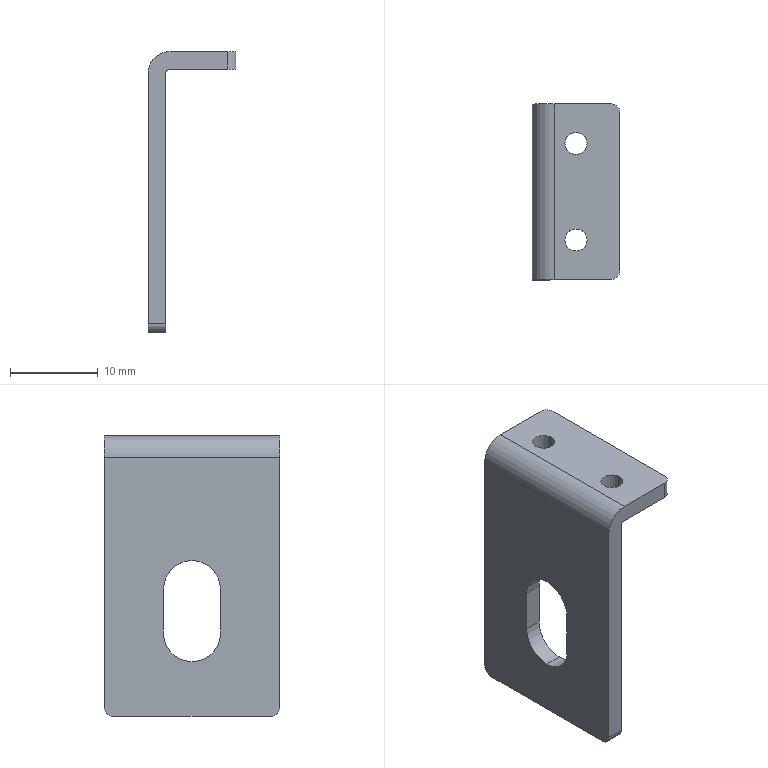Part | SolidWorks | features BaseBody 1, HoleWzd 1 | 1 solid | 23 faces | box 10 x 20 x 32 mm | volume 1421 mm3 | cylinder 13 | plane 10 | commonest cylinder face diameters 2 x4 2.51 x4 6.5 x3 1 x1 5 x1
STEP:
#1=CARTESIAN_POINT('',(4.255,15.5,0.));
#2=VERTEX_POINT('',#1);
#3=CARTESIAN_POINT('',(1.745,15.5,0.));
#4=VERTEX_POINT('',#3);
#5=CARTESIAN_POINT('',(3.,15.5,0.));
#6=DIRECTION('',(0.,0.,-1.));
#7=DIRECTION('',(-1.,0.,0.));
#8=AXIS2_PLACEMENT_3D('',#5,#6,#7);
#9=CIRCLE('',#8,1.255);
#10=EDGE_CURVE('',#2,#4,#9,.T.);
#11=ORIENTED_EDGE('',*,*,#10,.T.);
#12=CARTESIAN_POINT('',(1.745,15.5,2.));
#13=VERTEX_POINT('',#12);
#14=CARTESIAN_POINT('',(1.745,15.5,2.));
#15=DIRECTION('',(0.,0.,1.));
#16=VECTOR('',#15,1000.);
#17=LINE('',#14,#16);
#18=EDGE_CURVE('',#4,#13,#17,.T.);
#19=ORIENTED_EDGE('',*,*,#18,.T.);
#20=CARTESIAN_POINT('',(4.255,15.5,2.));
#21=VERTEX_POINT('',#20);
#22=CARTESIAN_POINT('',(3.,15.5,2.));
#23=DIRECTION('',(0.,0.,1.));
#24=DIRECTION('',(1.,0.,0.));
#25=AXIS2_PLACEMENT_3D('',#22,#23,#24);
#26=CIRCLE('',#25,1.255);
#27=EDGE_CURVE('',#13,#21,#26,.T.);
#28=ORIENTED_EDGE('',*,*,#27,.T.);
#29=CARTESIAN_POINT('',(4.255,15.5,2.));
#30=DIRECTION('',(0.,0.,1.));
#31=VECTOR('',#30,1000.);
#32=LINE('',#29,#31);
#33=EDGE_CURVE('',#2,#21,#32,.T.);
#34=ORIENTED_EDGE('',*,*,#33,.F.);
#35=EDGE_LOOP('',(#11,#19,#28,#34));
#36=FACE_OUTER_BOUND('',#35,.T.);
#37=CARTESIAN_POINT('',(3.,15.5,2.));
#38=DIRECTION('',(0.,0.,1.));
#39=DIRECTION('',(1.,0.,0.));
#40=AXIS2_PLACEMENT_3D('',#37,#38,#39);
#41=CYLINDRICAL_SURFACE('',#40,1.255);
#42=ADVANCED_FACE('',(#36),#41,.F.);
#43=CARTESIAN_POINT('',(4.255,4.5,0.));
#44=VERTEX_POINT('',#43);
#45=CARTESIAN_POINT('',(1.745,4.5,0.));
#46=VERTEX_POINT('',#45);
#47=CARTESIAN_POINT('',(3.,4.5,0.));
#48=DIRECTION('',(0.,0.,-1.));
#49=DIRECTION('',(-1.,0.,0.));
#50=AXIS2_PLACEMENT_3D('',#47,#48,#49);
#51=CIRCLE('',#50,1.255);
#52=EDGE_CURVE('',#44,#46,#51,.T.);
#53=ORIENTED_EDGE('',*,*,#52,.T.);
#54=CARTESIAN_POINT('',(1.745,4.5,2.));
#55=VERTEX_POINT('',#54);
#56=CARTESIAN_POINT('',(1.745,4.5,2.));
#57=DIRECTION('',(0.,0.,1.));
#58=VECTOR('',#57,1000.);
#59=LINE('',#56,#58);
#60=EDGE_CURVE('',#46,#55,#59,.T.);
#61=ORIENTED_EDGE('',*,*,#60,.T.);
#62=CARTESIAN_POINT('',(4.255,4.5,2.));
#63=VERTEX_POINT('',#62);
#64=CARTESIAN_POINT('',(3.,4.5,2.));
#65=DIRECTION('',(0.,0.,1.));
#66=DIRECTION('',(1.,0.,0.));
#67=AXIS2_PLACEMENT_3D('',#64,#65,#66);
#68=CIRCLE('',#67,1.255);
#69=EDGE_CURVE('',#55,#63,#68,.T.);
#70=ORIENTED_EDGE('',*,*,#69,.T.);
#71=CARTESIAN_POINT('',(4.255,4.5,2.));
#72=DIRECTION('',(0.,0.,1.));
#73=VECTOR('',#72,1000.);
#74=LINE('',#71,#73);
#75=EDGE_CURVE('',#44,#63,#74,.T.);
#76=ORIENTED_EDGE('',*,*,#75,.F.);
#77=EDGE_LOOP('',(#53,#61,#70,#76));
#78=FACE_OUTER_BOUND('',#77,.T.);
#79=CARTESIAN_POINT('',(3.,4.5,2.));
#80=DIRECTION('',(0.,0.,1.));
#81=DIRECTION('',(1.,0.,0.));
#82=AXIS2_PLACEMENT_3D('',#79,#80,#81);
#83=CYLINDRICAL_SURFACE('',#82,1.255);
#84=ADVANCED_FACE('',(#78),#83,.F.);
#85=CARTESIAN_POINT('',(-2.,10.,-23.75));
#86=VERTEX_POINT('',#85);
#87=CARTESIAN_POINT('',(-2.,13.25,-20.5));
#88=VERTEX_POINT('',#87);
#89=CARTESIAN_POINT('',(-2.,10.,-20.5));
#90=DIRECTION('',(1.,0.,0.));
#91=DIRECTION('',(0.,0.,-1.));
#92=AXIS2_PLACEMENT_3D('',#89,#90,#91);
#93=CIRCLE('',#92,3.25);
#94=EDGE_CURVE('',#86,#88,#93,.T.);
#95=ORIENTED_EDGE('',*,*,#94,.F.);
#96=CARTESIAN_POINT('',(0.,10.,-23.75));
#97=VERTEX_POINT('',#96);
#98=CARTESIAN_POINT('',(0.,10.,-23.75));
#99=DIRECTION('',(1.,0.,0.));
#100=VECTOR('',#99,1000.);
#101=LINE('',#98,#100);
#102=EDGE_CURVE('',#86,#97,#101,.T.);
#103=ORIENTED_EDGE('',*,*,#102,.T.);
#104=CARTESIAN_POINT('',(0.,13.25,-20.5));
#105=VERTEX_POINT('',#104);
#106=CARTESIAN_POINT('',(0.,10.,-20.5));
#107=DIRECTION('',(-1.,0.,0.));
#108=DIRECTION('',(0.,0.,-1.));
#109=AXIS2_PLACEMENT_3D('',#106,#107,#108);
#110=CIRCLE('',#109,3.25);
#111=EDGE_CURVE('',#105,#97,#110,.T.);
#112=ORIENTED_EDGE('',*,*,#111,.F.);
#113=CARTESIAN_POINT('',(0.,13.25,-20.5));
#114=DIRECTION('',(1.,0.,0.));
#115=VECTOR('',#114,1000.);
#116=LINE('',#113,#115);
#117=EDGE_CURVE('',#88,#105,#116,.T.);
#118=ORIENTED_EDGE('',*,*,#117,.F.);
#119=EDGE_LOOP('',(#95,#103,#112,#118));
#120=FACE_OUTER_BOUND('',#119,.T.);
#121=CARTESIAN_POINT('',(0.,10.,-20.5));
#122=DIRECTION('',(1.,0.,0.));
#123=DIRECTION('',(0.,0.,-1.));
#124=AXIS2_PLACEMENT_3D('',#121,#122,#123);
#125=CYLINDRICAL_SURFACE('',#124,3.25);
#126=ADVANCED_FACE('',(#120),#125,.F.);
#127=CARTESIAN_POINT('',(3.,15.5,2.));
#128=DIRECTION('',(0.,0.,1.));
#129=DIRECTION('',(1.,0.,0.));
#130=AXIS2_PLACEMENT_3D('',#127,#128,#129);
#131=CIRCLE('',#130,1.255);
#132=EDGE_CURVE('',#21,#13,#131,.T.);
#133=ORIENTED_EDGE('',*,*,#132,.F.);
#134=ORIENTED_EDGE('',*,*,#27,.F.);
#135=EDGE_LOOP('',(#133,#134));
#136=FACE_BOUND('',#135,.T.);
#137=CARTESIAN_POINT('',(8.,1.,2.));
#138=VERTEX_POINT('',#137);
#139=CARTESIAN_POINT('',(7.,0.,2.));
#140=VERTEX_POINT('',#139);
#141=CARTESIAN_POINT('',(7.,1.,2.));
#142=DIRECTION('',(0.,0.,-1.));
#143=DIRECTION('',(1.,0.,0.));
#144=AXIS2_PLACEMENT_3D('',#141,#142,#143);
#145=CIRCLE('',#144,1.);
#146=EDGE_CURVE('',#138,#140,#145,.T.);
#147=ORIENTED_EDGE('',*,*,#146,.F.);
#148=CARTESIAN_POINT('',(8.,19.,2.));
#149=VERTEX_POINT('',#148);
#150=CARTESIAN_POINT('',(8.,20.,2.));
#151=DIRECTION('',(0.,-1.,0.));
#152=VECTOR('',#151,1000.);
#153=LINE('',#150,#152);
#154=EDGE_CURVE('',#149,#138,#153,.T.);
#155=ORIENTED_EDGE('',*,*,#154,.F.);
#156=CARTESIAN_POINT('',(7.,20.,2.));
#157=VERTEX_POINT('',#156);
#158=CARTESIAN_POINT('',(7.,19.,2.));
#159=DIRECTION('',(0.,0.,-1.));
#160=DIRECTION('',(1.,0.,0.));
#161=AXIS2_PLACEMENT_3D('',#158,#159,#160);
#162=CIRCLE('',#161,1.);
#163=EDGE_CURVE('',#157,#149,#162,.T.);
#164=ORIENTED_EDGE('',*,*,#163,.F.);
#165=CARTESIAN_POINT('',(0.5,20.,2.));
#166=VERTEX_POINT('',#165);
#167=CARTESIAN_POINT('',(-2.,20.,2.));
#168=DIRECTION('',(1.,0.,0.));
#169=VECTOR('',#168,1000.);
#170=LINE('',#167,#169);
#171=EDGE_CURVE('',#166,#157,#170,.T.);
#172=ORIENTED_EDGE('',*,*,#171,.F.);
#173=CARTESIAN_POINT('',(0.5,0.,2.));
#174=VERTEX_POINT('',#173);
#175=CARTESIAN_POINT('',(0.5,20.,2.));
#176=DIRECTION('',(0.,1.,0.));
#177=VECTOR('',#176,1000.);
#178=LINE('',#175,#177);
#179=EDGE_CURVE('',#174,#166,#178,.T.);
#180=ORIENTED_EDGE('',*,*,#179,.F.);
#181=CARTESIAN_POINT('',(0.5,0.,2.));
#182=DIRECTION('',(-1.,0.,0.));
#183=VECTOR('',#182,1000.);
#184=LINE('',#181,#183);
#185=EDGE_CURVE('',#140,#174,#184,.T.);
#186=ORIENTED_EDGE('',*,*,#185,.F.);
#187=EDGE_LOOP('',(#147,#155,#164,#172,#180,#186));
#188=FACE_OUTER_BOUND('',#187,.T.);
#189=CARTESIAN_POINT('',(3.,4.5,2.));
#190=DIRECTION('',(0.,0.,1.));
#191=DIRECTION('',(1.,0.,0.));
#192=AXIS2_PLACEMENT_3D('',#189,#190,#191);
#193=CIRCLE('',#192,1.255);
#194=EDGE_CURVE('',#63,#55,#193,.T.);
#195=ORIENTED_EDGE('',*,*,#194,.F.);
#196=ORIENTED_EDGE('',*,*,#69,.F.);
#197=EDGE_LOOP('',(#195,#196));
#198=FACE_BOUND('',#197,.T.);
#199=CARTESIAN_POINT('',(0.,20.,2.));
#200=DIRECTION('',(0.,0.,-1.));
#201=DIRECTION('',(-1.,0.,0.));
#202=AXIS2_PLACEMENT_3D('',#199,#200,#201);
#203=PLANE('',#202);
#204=ADVANCED_FACE('',(#136,#188,#198),#203,.F.);
#205=CARTESIAN_POINT('',(0.,0.,-0.5));
#206=VERTEX_POINT('',#205);
#207=CARTESIAN_POINT('',(0.,0.,-29.));
#208=VERTEX_POINT('',#207);
#209=CARTESIAN_POINT('',(0.,0.,-30.));
#210=DIRECTION('',(0.,0.,-1.));
#211=VECTOR('',#210,1000.);
#212=LINE('',#209,#211);
#213=EDGE_CURVE('',#206,#208,#212,.T.);
#214=ORIENTED_EDGE('',*,*,#213,.T.);
#215=CARTESIAN_POINT('',(0.,1.,-30.));
#216=VERTEX_POINT('',#215);
#217=CARTESIAN_POINT('',(0.,1.,-29.));
#218=DIRECTION('',(-1.,0.,0.));
#219=DIRECTION('',(0.,0.,-1.));
#220=AXIS2_PLACEMENT_3D('',#217,#218,#219);
#221=CIRCLE('',#220,1.);
#222=EDGE_CURVE('',#216,#208,#221,.T.);
#223=ORIENTED_EDGE('',*,*,#222,.F.);
#224=CARTESIAN_POINT('',(0.,19.,-30.));
#225=VERTEX_POINT('',#224);
#226=CARTESIAN_POINT('',(0.,20.,-30.));
#227=DIRECTION('',(0.,1.,0.));
#228=VECTOR('',#227,1000.);
#229=LINE('',#226,#228);
#230=EDGE_CURVE('',#216,#225,#229,.T.);
#231=ORIENTED_EDGE('',*,*,#230,.T.);
#232=CARTESIAN_POINT('',(0.,20.,-29.));
#233=VERTEX_POINT('',#232);
#234=CARTESIAN_POINT('',(0.,19.,-29.));
#235=DIRECTION('',(-1.,0.,0.));
#236=DIRECTION('',(0.,0.,1.));
#237=AXIS2_PLACEMENT_3D('',#234,#235,#236);
#238=CIRCLE('',#237,1.);
#239=EDGE_CURVE('',#233,#225,#238,.T.);
#240=ORIENTED_EDGE('',*,*,#239,.F.);
#241=CARTESIAN_POINT('',(0.,20.,-0.5));
#242=VERTEX_POINT('',#241);
#243=CARTESIAN_POINT('',(0.,20.,-30.));
#244=DIRECTION('',(0.,0.,1.));
#245=VECTOR('',#244,1000.);
#246=LINE('',#243,#245);
#247=EDGE_CURVE('',#233,#242,#246,.T.);
#248=ORIENTED_EDGE('',*,*,#247,.T.);
#249=CARTESIAN_POINT('',(0.,20.,-0.5));
#250=DIRECTION('',(0.,-1.,0.));
#251=VECTOR('',#250,1000.);
#252=LINE('',#249,#251);
#253=EDGE_CURVE('',#242,#206,#252,.T.);
#254=ORIENTED_EDGE('',*,*,#253,.T.);
#255=EDGE_LOOP('',(#214,#223,#231,#240,#248,#254));
#256=FACE_OUTER_BOUND('',#255,.T.);
#257=CARTESIAN_POINT('',(0.,6.75,-20.5));
#258=VERTEX_POINT('',#257);
#259=CARTESIAN_POINT('',(0.,6.75,-15.5));
#260=VERTEX_POINT('',#259);
#261=CARTESIAN_POINT('',(0.,6.75,-30.));
#262=DIRECTION('',(0.,0.,1.));
#263=VECTOR('',#262,1000.);
#264=LINE('',#261,#263);
#265=EDGE_CURVE('',#258,#260,#264,.T.);
#266=ORIENTED_EDGE('',*,*,#265,.T.);
#267=CARTESIAN_POINT('',(0.,13.25,-15.5));
#268=VERTEX_POINT('',#267);
#269=CARTESIAN_POINT('',(0.,10.,-15.5));
#270=DIRECTION('',(-1.,0.,0.));
#271=DIRECTION('',(0.,0.,-1.));
#272=AXIS2_PLACEMENT_3D('',#269,#270,#271);
#273=CIRCLE('',#272,3.25);
#274=EDGE_CURVE('',#260,#268,#273,.T.);
#275=ORIENTED_EDGE('',*,*,#274,.T.);
#276=CARTESIAN_POINT('',(0.,13.25,-30.));
#277=DIRECTION('',(0.,0.,-1.));
#278=VECTOR('',#277,1000.);
#279=LINE('',#276,#278);
#280=EDGE_CURVE('',#268,#105,#279,.T.);
#281=ORIENTED_EDGE('',*,*,#280,.T.);
#282=ORIENTED_EDGE('',*,*,#111,.T.);
#283=CARTESIAN_POINT('',(0.,10.,-20.5));
#284=DIRECTION('',(-1.,0.,0.));
#285=DIRECTION('',(0.,0.,-1.));
#286=AXIS2_PLACEMENT_3D('',#283,#284,#285);
#287=CIRCLE('',#286,3.25);
#288=EDGE_CURVE('',#97,#258,#287,.T.);
#289=ORIENTED_EDGE('',*,*,#288,.T.);
#290=EDGE_LOOP('',(#266,#275,#281,#282,#289));
#291=FACE_BOUND('',#290,.T.);
#292=CARTESIAN_POINT('',(0.,20.,-30.));
#293=DIRECTION('',(1.,0.,0.));
#294=DIRECTION('',(0.,0.,-1.));
#295=AXIS2_PLACEMENT_3D('',#292,#293,#294);
#296=PLANE('',#295);
#297=ADVANCED_FACE('',(#256,#291),#296,.T.);
#298=ORIENTED_EDGE('',*,*,#213,.F.);
#299=CARTESIAN_POINT('',(0.5,0.,0.));
#300=VERTEX_POINT('',#299);
#301=CARTESIAN_POINT('',(0.5,0.,-0.5));
#302=DIRECTION('',(0.,1.,0.));
#303=DIRECTION('',(0.,0.,-1.));
#304=AXIS2_PLACEMENT_3D('',#301,#302,#303);
#305=CIRCLE('',#304,0.5);
#306=EDGE_CURVE('',#206,#300,#305,.T.);
#307=ORIENTED_EDGE('',*,*,#306,.T.);
#308=CARTESIAN_POINT('',(7.,0.,0.));
#309=VERTEX_POINT('',#308);
#310=CARTESIAN_POINT('',(0.,0.,0.));
#311=DIRECTION('',(-1.,0.,0.));
#312=VECTOR('',#311,1000.);
#313=LINE('',#310,#312);
#314=EDGE_CURVE('',#309,#300,#313,.T.);
#315=ORIENTED_EDGE('',*,*,#314,.F.);
#316=CARTESIAN_POINT('',(7.,0.,-0.5));
#317=DIRECTION('',(0.,0.,1.));
#318=VECTOR('',#317,1000.);
#319=LINE('',#316,#318);
#320=EDGE_CURVE('',#309,#140,#319,.T.);
#321=ORIENTED_EDGE('',*,*,#320,.T.);
#322=ORIENTED_EDGE('',*,*,#185,.T.);
#323=CARTESIAN_POINT('',(-2.,0.,-0.5));
#324=VERTEX_POINT('',#323);
#325=CARTESIAN_POINT('',(0.5,0.,-0.5));
#326=DIRECTION('',(0.,-1.,0.));
#327=DIRECTION('',(0.,0.,-1.));
#328=AXIS2_PLACEMENT_3D('',#325,#326,#327);
#329=CIRCLE('',#328,2.5);
#330=EDGE_CURVE('',#174,#324,#329,.T.);
#331=ORIENTED_EDGE('',*,*,#330,.T.);
#332=CARTESIAN_POINT('',(-2.,0.,-29.));
#333=VERTEX_POINT('',#332);
#334=CARTESIAN_POINT('',(-2.,0.,2.));
#335=DIRECTION('',(0.,0.,-1.));
#336=VECTOR('',#335,1000.);
#337=LINE('',#334,#336);
#338=EDGE_CURVE('',#324,#333,#337,.T.);
#339=ORIENTED_EDGE('',*,*,#338,.T.);
#340=CARTESIAN_POINT('',(0.5,0.,-29.));
#341=DIRECTION('',(1.,0.,0.));
#342=VECTOR('',#341,1000.);
#343=LINE('',#340,#342);
#344=EDGE_CURVE('',#333,#208,#343,.T.);
#345=ORIENTED_EDGE('',*,*,#344,.T.);
#346=EDGE_LOOP('',(#298,#307,#315,#321,#322,#331,#339,#345));
#347=FACE_OUTER_BOUND('',#346,.T.);
#348=CARTESIAN_POINT('',(0.5,0.,2.));
#349=DIRECTION('',(0.,-1.,0.));
#350=DIRECTION('',(0.,0.,-1.));
#351=AXIS2_PLACEMENT_3D('',#348,#349,#350);
#352=PLANE('',#351);
#353=ADVANCED_FACE('',(#347),#352,.T.);
#354=ORIENTED_EDGE('',*,*,#253,.F.);
#355=CARTESIAN_POINT('',(0.5,20.,0.));
#356=VERTEX_POINT('',#355);
#357=CARTESIAN_POINT('',(0.5,20.,-0.5));
#358=DIRECTION('',(0.,-1.,0.));
#359=DIRECTION('',(0.,0.,-1.));
#360=AXIS2_PLACEMENT_3D('',#357,#358,#359);
#361=CIRCLE('',#360,0.5);
#362=EDGE_CURVE('',#356,#242,#361,.T.);
#363=ORIENTED_EDGE('',*,*,#362,.F.);
#364=CARTESIAN_POINT('',(0.5,20.,0.));
#365=DIRECTION('',(0.,1.,0.));
#366=VECTOR('',#365,1000.);
#367=LINE('',#364,#366);
#368=EDGE_CURVE('',#300,#356,#367,.T.);
#369=ORIENTED_EDGE('',*,*,#368,.F.);
#370=ORIENTED_EDGE('',*,*,#306,.F.);
#371=EDGE_LOOP('',(#354,#363,#369,#370));
#372=FACE_OUTER_BOUND('',#371,.T.);
#373=CARTESIAN_POINT('',(0.5,20.,-0.5));
#374=DIRECTION('',(0.,-1.,0.));
#375=DIRECTION('',(0.,0.,-1.));
#376=AXIS2_PLACEMENT_3D('',#373,#374,#375);
#377=CYLINDRICAL_SURFACE('',#376,0.5);
#378=ADVANCED_FACE('',(#372),#377,.F.);
#379=CARTESIAN_POINT('',(-2.,20.,-29.));
#380=VERTEX_POINT('',#379);
#381=CARTESIAN_POINT('',(0.5,20.,-29.));
#382=DIRECTION('',(1.,0.,0.));
#383=VECTOR('',#382,1000.);
#384=LINE('',#381,#383);
#385=EDGE_CURVE('',#380,#233,#384,.T.);
#386=ORIENTED_EDGE('',*,*,#385,.F.);
#387=CARTESIAN_POINT('',(-2.,20.,-0.5));
#388=VERTEX_POINT('',#387);
#389=CARTESIAN_POINT('',(-2.,20.,-0.5));
#390=DIRECTION('',(0.,0.,-1.));
#391=VECTOR('',#390,1000.);
#392=LINE('',#389,#391);
#393=EDGE_CURVE('',#388,#380,#392,.T.);
#394=ORIENTED_EDGE('',*,*,#393,.F.);
#395=CARTESIAN_POINT('',(0.5,20.,-0.5));
#396=DIRECTION('',(0.,1.,0.));
#397=DIRECTION('',(0.,0.,-1.));
#398=AXIS2_PLACEMENT_3D('',#395,#396,#397);
#399=CIRCLE('',#398,2.5);
#400=EDGE_CURVE('',#388,#166,#399,.T.);
#401=ORIENTED_EDGE('',*,*,#400,.T.);
#402=ORIENTED_EDGE('',*,*,#171,.T.);
#403=CARTESIAN_POINT('',(7.,20.,0.));
#404=VERTEX_POINT('',#403);
#405=CARTESIAN_POINT('',(7.,20.,-0.5));
#406=DIRECTION('',(0.,0.,-1.));
#407=VECTOR('',#406,1000.);
#408=LINE('',#405,#407);
#409=EDGE_CURVE('',#157,#404,#408,.T.);
#410=ORIENTED_EDGE('',*,*,#409,.T.);
#411=CARTESIAN_POINT('',(0.,20.,0.));
#412=DIRECTION('',(1.,0.,0.));
#413=VECTOR('',#412,1000.);
#414=LINE('',#411,#413);
#415=EDGE_CURVE('',#356,#404,#414,.T.);
#416=ORIENTED_EDGE('',*,*,#415,.F.);
#417=ORIENTED_EDGE('',*,*,#362,.T.);
#418=ORIENTED_EDGE('',*,*,#247,.F.);
#419=EDGE_LOOP('',(#386,#394,#401,#402,#410,#416,#417,#418));
#420=FACE_OUTER_BOUND('',#419,.T.);
#421=CARTESIAN_POINT('',(0.5,20.,-0.5));
#422=DIRECTION('',(0.,-1.,0.));
#423=DIRECTION('',(0.,0.,-1.));
#424=AXIS2_PLACEMENT_3D('',#421,#422,#423);
#425=PLANE('',#424);
#426=ADVANCED_FACE('',(#420),#425,.F.);
#427=ORIENTED_EDGE('',*,*,#230,.F.);
#428=CARTESIAN_POINT('',(-2.,1.,-30.));
#429=VERTEX_POINT('',#428);
#430=CARTESIAN_POINT('',(-2.,1.,-30.));
#431=DIRECTION('',(-1.,0.,0.));
#432=VECTOR('',#431,1000.);
#433=LINE('',#430,#432);
#434=EDGE_CURVE('',#216,#429,#433,.T.);
#435=ORIENTED_EDGE('',*,*,#434,.T.);
#436=CARTESIAN_POINT('',(-2.,19.,-30.));
#437=VERTEX_POINT('',#436);
#438=CARTESIAN_POINT('',(-2.,20.,-30.));
#439=DIRECTION('',(0.,1.,0.));
#440=VECTOR('',#439,1000.);
#441=LINE('',#438,#440);
#442=EDGE_CURVE('',#429,#437,#441,.T.);
#443=ORIENTED_EDGE('',*,*,#442,.T.);
#444=CARTESIAN_POINT('',(-2.,19.,-30.));
#445=DIRECTION('',(1.,0.,0.));
#446=VECTOR('',#445,1000.);
#447=LINE('',#444,#446);
#448=EDGE_CURVE('',#437,#225,#447,.T.);
#449=ORIENTED_EDGE('',*,*,#448,.T.);
#450=EDGE_LOOP('',(#427,#435,#443,#449));
#451=FACE_OUTER_BOUND('',#450,.T.);
#452=CARTESIAN_POINT('',(-2.,20.,-30.));
#453=DIRECTION('',(0.,0.,-1.));
#454=DIRECTION('',(-1.,0.,0.));
#455=AXIS2_PLACEMENT_3D('',#452,#453,#454);
#456=PLANE('',#455);
#457=ADVANCED_FACE('',(#451),#456,.T.);
#458=CARTESIAN_POINT('',(-2.,13.25,-15.5));
#459=VERTEX_POINT('',#458);
#460=CARTESIAN_POINT('',(0.,13.25,-15.5));
#461=DIRECTION('',(-1.,0.,0.));
#462=VECTOR('',#461,1000.);
#463=LINE('',#460,#462);
#464=EDGE_CURVE('',#268,#459,#463,.T.);
#465=ORIENTED_EDGE('',*,*,#464,.F.);
#466=ORIENTED_EDGE('',*,*,#274,.F.);
#467=CARTESIAN_POINT('',(-2.,6.75,-15.5));
#468=VERTEX_POINT('',#467);
#469=CARTESIAN_POINT('',(0.,6.75,-15.5));
#470=DIRECTION('',(1.,0.,0.));
#471=VECTOR('',#470,1000.);
#472=LINE('',#469,#471);
#473=EDGE_CURVE('',#468,#260,#472,.T.);
#474=ORIENTED_EDGE('',*,*,#473,.F.);
#475=CARTESIAN_POINT('',(-2.,10.,-15.5));
#476=DIRECTION('',(1.,0.,0.));
#477=DIRECTION('',(0.,0.,-1.));
#478=AXIS2_PLACEMENT_3D('',#475,#476,#477);
#479=CIRCLE('',#478,3.25);
#480=EDGE_CURVE('',#459,#468,#479,.T.);
#481=ORIENTED_EDGE('',*,*,#480,.F.);
#482=EDGE_LOOP('',(#465,#466,#474,#481));
#483=FACE_OUTER_BOUND('',#482,.T.);
#484=CARTESIAN_POINT('',(0.,10.,-15.5));
#485=DIRECTION('',(1.,0.,0.));
#486=DIRECTION('',(0.,0.,-1.));
#487=AXIS2_PLACEMENT_3D('',#484,#485,#486);
#488=CYLINDRICAL_SURFACE('',#487,3.25);
#489=ADVANCED_FACE('',(#483),#488,.F.);
#490=ORIENTED_EDGE('',*,*,#265,.F.);
#491=CARTESIAN_POINT('',(-2.,6.75,-20.5));
#492=VERTEX_POINT('',#491);
#493=CARTESIAN_POINT('',(0.,6.75,-20.5));
#494=DIRECTION('',(1.,0.,0.));
#495=VECTOR('',#494,1000.);
#496=LINE('',#493,#495);
#497=EDGE_CURVE('',#492,#258,#496,.T.);
#498=ORIENTED_EDGE('',*,*,#497,.F.);
#499=CARTESIAN_POINT('',(-2.,6.75,-20.5));
#500=DIRECTION('',(0.,0.,-1.));
#501=VECTOR('',#500,1000.);
#502=LINE('',#499,#501);
#503=EDGE_CURVE('',#468,#492,#502,.T.);
#504=ORIENTED_EDGE('',*,*,#503,.F.);
#505=ORIENTED_EDGE('',*,*,#473,.T.);
#506=EDGE_LOOP('',(#490,#498,#504,#505));
#507=FACE_OUTER_BOUND('',#506,.T.);
#508=CARTESIAN_POINT('',(0.,6.75,-20.5));
#509=DIRECTION('',(0.,-1.,0.));
#510=DIRECTION('',(0.,0.,-1.));
#511=AXIS2_PLACEMENT_3D('',#508,#509,#510);
#512=PLANE('',#511);
#513=ADVANCED_FACE('',(#507),#512,.F.);
#514=ORIENTED_EDGE('',*,*,#102,.F.);
#515=CARTESIAN_POINT('',(-2.,10.,-20.5));
#516=DIRECTION('',(1.,0.,0.));
#517=DIRECTION('',(0.,0.,-1.));
#518=AXIS2_PLACEMENT_3D('',#515,#516,#517);
#519=CIRCLE('',#518,3.25);
#520=EDGE_CURVE('',#492,#86,#519,.T.);
#521=ORIENTED_EDGE('',*,*,#520,.F.);
#522=ORIENTED_EDGE('',*,*,#497,.T.);
#523=ORIENTED_EDGE('',*,*,#288,.F.);
#524=EDGE_LOOP('',(#514,#521,#522,#523));
#525=FACE_OUTER_BOUND('',#524,.T.);
#526=CARTESIAN_POINT('',(0.,10.,-20.5));
#527=DIRECTION('',(1.,0.,0.));
#528=DIRECTION('',(0.,0.,-1.));
#529=AXIS2_PLACEMENT_3D('',#526,#527,#528);
#530=CYLINDRICAL_SURFACE('',#529,3.25);
#531=ADVANCED_FACE('',(#525),#530,.F.);
#532=CARTESIAN_POINT('',(-2.,13.25,-20.5));
#533=DIRECTION('',(0.,0.,1.));
#534=VECTOR('',#533,1000.);
#535=LINE('',#532,#534);
#536=EDGE_CURVE('',#88,#459,#535,.T.);
#537=ORIENTED_EDGE('',*,*,#536,.F.);
#538=ORIENTED_EDGE('',*,*,#117,.T.);
#539=ORIENTED_EDGE('',*,*,#280,.F.);
#540=ORIENTED_EDGE('',*,*,#464,.T.);
#541=EDGE_LOOP('',(#537,#538,#539,#540));
#542=FACE_OUTER_BOUND('',#541,.T.);
#543=CARTESIAN_POINT('',(-2.,13.25,-20.5));
#544=DIRECTION('',(0.,1.,0.));
#545=DIRECTION('',(-1.,0.,0.));
#546=AXIS2_PLACEMENT_3D('',#543,#544,#545);
#547=PLANE('',#546);
#548=ADVANCED_FACE('',(#542),#547,.F.);
#549=ORIENTED_EDGE('',*,*,#222,.T.);
#550=ORIENTED_EDGE('',*,*,#344,.F.);
#551=CARTESIAN_POINT('',(-2.,1.,-29.));
#552=DIRECTION('',(1.,0.,0.));
#553=DIRECTION('',(0.,0.,-1.));
#554=AXIS2_PLACEMENT_3D('',#551,#552,#553);
#555=CIRCLE('',#554,1.);
#556=EDGE_CURVE('',#333,#429,#555,.T.);
#557=ORIENTED_EDGE('',*,*,#556,.T.);
#558=ORIENTED_EDGE('',*,*,#434,.F.);
#559=EDGE_LOOP('',(#549,#550,#557,#558));
#560=FACE_OUTER_BOUND('',#559,.T.);
#561=CARTESIAN_POINT('',(0.5,1.,-29.));
#562=DIRECTION('',(1.,0.,0.));
#563=DIRECTION('',(0.,0.,-1.));
#564=AXIS2_PLACEMENT_3D('',#561,#562,#563);
#565=CYLINDRICAL_SURFACE('',#564,1.);
#566=ADVANCED_FACE('',(#560),#565,.T.);
#567=CARTESIAN_POINT('',(-2.,19.,-29.));
#568=DIRECTION('',(1.,0.,0.));
#569=DIRECTION('',(0.,0.,1.));
#570=AXIS2_PLACEMENT_3D('',#567,#568,#569);
#571=CIRCLE('',#570,1.);
#572=EDGE_CURVE('',#437,#380,#571,.T.);
#573=ORIENTED_EDGE('',*,*,#572,.F.);
#574=ORIENTED_EDGE('',*,*,#442,.F.);
#575=ORIENTED_EDGE('',*,*,#556,.F.);
#576=ORIENTED_EDGE('',*,*,#338,.F.);
#577=CARTESIAN_POINT('',(-2.,20.,-0.5));
#578=DIRECTION('',(0.,-1.,0.));
#579=VECTOR('',#578,1000.);
#580=LINE('',#577,#579);
#581=EDGE_CURVE('',#388,#324,#580,.T.);
#582=ORIENTED_EDGE('',*,*,#581,.F.);
#583=ORIENTED_EDGE('',*,*,#393,.T.);
#584=EDGE_LOOP('',(#573,#574,#575,#576,#582,#583));
#585=FACE_OUTER_BOUND('',#584,.T.);
#586=ORIENTED_EDGE('',*,*,#520,.T.);
#587=ORIENTED_EDGE('',*,*,#94,.T.);
#588=ORIENTED_EDGE('',*,*,#536,.T.);
#589=ORIENTED_EDGE('',*,*,#480,.T.);
#590=ORIENTED_EDGE('',*,*,#503,.T.);
#591=EDGE_LOOP('',(#586,#587,#588,#589,#590));
#592=FACE_BOUND('',#591,.T.);
#593=CARTESIAN_POINT('',(-2.,20.,-30.));
#594=DIRECTION('',(1.,0.,0.));
#595=DIRECTION('',(0.,0.,-1.));
#596=AXIS2_PLACEMENT_3D('',#593,#594,#595);
#597=PLANE('',#596);
#598=ADVANCED_FACE('',(#585,#592),#597,.F.);
#599=ORIENTED_EDGE('',*,*,#10,.F.);
#600=CARTESIAN_POINT('',(3.,15.5,0.));
#601=DIRECTION('',(0.,0.,-1.));
#602=DIRECTION('',(-1.,0.,0.));
#603=AXIS2_PLACEMENT_3D('',#600,#601,#602);
#604=CIRCLE('',#603,1.255);
#605=EDGE_CURVE('',#4,#2,#604,.T.);
#606=ORIENTED_EDGE('',*,*,#605,.F.);
#607=EDGE_LOOP('',(#599,#606));
#608=FACE_BOUND('',#607,.T.);
#609=ORIENTED_EDGE('',*,*,#52,.F.);
#610=CARTESIAN_POINT('',(3.,4.5,0.));
#611=DIRECTION('',(0.,0.,-1.));
#612=DIRECTION('',(-1.,0.,0.));
#613=AXIS2_PLACEMENT_3D('',#610,#611,#612);
#614=CIRCLE('',#613,1.255);
#615=EDGE_CURVE('',#46,#44,#614,.T.);
#616=ORIENTED_EDGE('',*,*,#615,.F.);
#617=EDGE_LOOP('',(#609,#616));
#618=FACE_BOUND('',#617,.T.);
#619=ORIENTED_EDGE('',*,*,#415,.T.);
#620=CARTESIAN_POINT('',(8.,19.,0.));
#621=VERTEX_POINT('',#620);
#622=CARTESIAN_POINT('',(7.,19.,0.));
#623=DIRECTION('',(0.,0.,1.));
#624=DIRECTION('',(1.,0.,0.));
#625=AXIS2_PLACEMENT_3D('',#622,#623,#624);
#626=CIRCLE('',#625,1.);
#627=EDGE_CURVE('',#621,#404,#626,.T.);
#628=ORIENTED_EDGE('',*,*,#627,.F.);
#629=CARTESIAN_POINT('',(8.,1.,0.));
#630=VERTEX_POINT('',#629);
#631=CARTESIAN_POINT('',(8.,20.,0.));
#632=DIRECTION('',(0.,-1.,0.));
#633=VECTOR('',#632,1000.);
#634=LINE('',#631,#633);
#635=EDGE_CURVE('',#621,#630,#634,.T.);
#636=ORIENTED_EDGE('',*,*,#635,.T.);
#637=CARTESIAN_POINT('',(7.,1.,0.));
#638=DIRECTION('',(0.,0.,1.));
#639=DIRECTION('',(1.,0.,0.));
#640=AXIS2_PLACEMENT_3D('',#637,#638,#639);
#641=CIRCLE('',#640,1.);
#642=EDGE_CURVE('',#309,#630,#641,.T.);
#643=ORIENTED_EDGE('',*,*,#642,.F.);
#644=ORIENTED_EDGE('',*,*,#314,.T.);
#645=ORIENTED_EDGE('',*,*,#368,.T.);
#646=EDGE_LOOP('',(#619,#628,#636,#643,#644,#645));
#647=FACE_OUTER_BOUND('',#646,.T.);
#648=CARTESIAN_POINT('',(0.,20.,0.));
#649=DIRECTION('',(0.,0.,-1.));
#650=DIRECTION('',(-1.,0.,0.));
#651=AXIS2_PLACEMENT_3D('',#648,#649,#650);
#652=PLANE('',#651);
#653=ADVANCED_FACE('',(#608,#618,#647),#652,.T.);
#654=ORIENTED_EDGE('',*,*,#239,.T.);
#655=ORIENTED_EDGE('',*,*,#448,.F.);
#656=ORIENTED_EDGE('',*,*,#572,.T.);
#657=ORIENTED_EDGE('',*,*,#385,.T.);
#658=EDGE_LOOP('',(#654,#655,#656,#657));
#659=FACE_OUTER_BOUND('',#658,.T.);
#660=CARTESIAN_POINT('',(-2.,19.,-29.));
#661=DIRECTION('',(-1.,0.,0.));
#662=DIRECTION('',(0.,0.,1.));
#663=AXIS2_PLACEMENT_3D('',#660,#661,#662);
#664=CYLINDRICAL_SURFACE('',#663,1.);
#665=ADVANCED_FACE('',(#659),#664,.T.);
#666=ORIENTED_EDGE('',*,*,#400,.F.);
#667=ORIENTED_EDGE('',*,*,#581,.T.);
#668=ORIENTED_EDGE('',*,*,#330,.F.);
#669=ORIENTED_EDGE('',*,*,#179,.T.);
#670=EDGE_LOOP('',(#666,#667,#668,#669));
#671=FACE_OUTER_BOUND('',#670,.T.);
#672=CARTESIAN_POINT('',(0.5,20.,-0.5));
#673=DIRECTION('',(0.,-1.,0.));
#674=DIRECTION('',(0.,0.,-1.));
#675=AXIS2_PLACEMENT_3D('',#672,#673,#674);
#676=CYLINDRICAL_SURFACE('',#675,2.5);
#677=ADVANCED_FACE('',(#671),#676,.T.);
#678=ORIENTED_EDGE('',*,*,#635,.F.);
#679=CARTESIAN_POINT('',(8.,19.,0.));
#680=DIRECTION('',(0.,0.,1.));
#681=VECTOR('',#680,1000.);
#682=LINE('',#679,#681);
#683=EDGE_CURVE('',#621,#149,#682,.T.);
#684=ORIENTED_EDGE('',*,*,#683,.T.);
#685=ORIENTED_EDGE('',*,*,#154,.T.);
#686=CARTESIAN_POINT('',(8.,1.,0.));
#687=DIRECTION('',(0.,0.,-1.));
#688=VECTOR('',#687,1000.);
#689=LINE('',#686,#688);
#690=EDGE_CURVE('',#138,#630,#689,.T.);
#691=ORIENTED_EDGE('',*,*,#690,.T.);
#692=EDGE_LOOP('',(#678,#684,#685,#691));
#693=FACE_OUTER_BOUND('',#692,.T.);
#694=CARTESIAN_POINT('',(8.,20.,0.));
#695=DIRECTION('',(1.,0.,0.));
#696=DIRECTION('',(0.,0.,-1.));
#697=AXIS2_PLACEMENT_3D('',#694,#695,#696);
#698=PLANE('',#697);
#699=ADVANCED_FACE('',(#693),#698,.T.);
#700=ORIENTED_EDGE('',*,*,#146,.T.);
#701=ORIENTED_EDGE('',*,*,#320,.F.);
#702=ORIENTED_EDGE('',*,*,#642,.T.);
#703=ORIENTED_EDGE('',*,*,#690,.F.);
#704=EDGE_LOOP('',(#700,#701,#702,#703));
#705=FACE_OUTER_BOUND('',#704,.T.);
#706=CARTESIAN_POINT('',(7.,1.,-0.5));
#707=DIRECTION('',(0.,0.,1.));
#708=DIRECTION('',(1.,0.,0.));
#709=AXIS2_PLACEMENT_3D('',#706,#707,#708);
#710=CYLINDRICAL_SURFACE('',#709,1.);
#711=ADVANCED_FACE('',(#705),#710,.T.);
#712=ORIENTED_EDGE('',*,*,#163,.T.);
#713=ORIENTED_EDGE('',*,*,#683,.F.);
#714=ORIENTED_EDGE('',*,*,#627,.T.);
#715=ORIENTED_EDGE('',*,*,#409,.F.);
#716=EDGE_LOOP('',(#712,#713,#714,#715));
#717=FACE_OUTER_BOUND('',#716,.T.);
#718=CARTESIAN_POINT('',(7.,19.,0.));
#719=DIRECTION('',(0.,0.,1.));
#720=DIRECTION('',(1.,0.,0.));
#721=AXIS2_PLACEMENT_3D('',#718,#719,#720);
#722=CYLINDRICAL_SURFACE('',#721,1.);
#723=ADVANCED_FACE('',(#717),#722,.T.);
#724=ORIENTED_EDGE('',*,*,#60,.F.);
#725=ORIENTED_EDGE('',*,*,#615,.T.);
#726=ORIENTED_EDGE('',*,*,#75,.T.);
#727=ORIENTED_EDGE('',*,*,#194,.T.);
#728=EDGE_LOOP('',(#724,#725,#726,#727));
#729=FACE_OUTER_BOUND('',#728,.T.);
#730=CARTESIAN_POINT('',(3.,4.5,2.));
#731=DIRECTION('',(0.,0.,1.));
#732=DIRECTION('',(1.,0.,0.));
#733=AXIS2_PLACEMENT_3D('',#730,#731,#732);
#734=CYLINDRICAL_SURFACE('',#733,1.255);
#735=ADVANCED_FACE('',(#729),#734,.F.);
#736=ORIENTED_EDGE('',*,*,#18,.F.);
#737=ORIENTED_EDGE('',*,*,#605,.T.);
#738=ORIENTED_EDGE('',*,*,#33,.T.);
#739=ORIENTED_EDGE('',*,*,#132,.T.);
#740=EDGE_LOOP('',(#736,#737,#738,#739));
#741=FACE_OUTER_BOUND('',#740,.T.);
#742=CARTESIAN_POINT('',(3.,15.5,2.));
#743=DIRECTION('',(0.,0.,1.));
#744=DIRECTION('',(1.,0.,0.));
#745=AXIS2_PLACEMENT_3D('',#742,#743,#744);
#746=CYLINDRICAL_SURFACE('',#745,1.255);
#747=ADVANCED_FACE('',(#741),#746,.F.);
#748=CLOSED_SHELL('',(#42,#84,#126,#204,#297,#353,#378,#426,#457,#489,#513,#531,#548,#566,#598,#653,#665,#677,#699,#711,#723,#735,#747));
#749=MANIFOLD_SOLID_BREP('',#748);
#750=CARTESIAN_POINT('',(0.,0.,0.));
#751=DIRECTION('',(0.,0.,1.));
#752=DIRECTION('',(1.,0.,0.));
#753=AXIS2_PLACEMENT_3D('',#750,#751,#752);
#754=(LENGTH_UNIT()NAMED_UNIT(*)SI_UNIT(.MILLI.,.METRE.));
#755=UNCERTAINTY_MEASURE_WITH_UNIT(LENGTH_MEASURE(0.00001),#754,'','');
#756=(NAMED_UNIT(*)PLANE_ANGLE_UNIT()SI_UNIT($,.RADIAN.));
#757=(NAMED_UNIT(*)SI_UNIT($,.STERADIAN.)SOLID_ANGLE_UNIT());
#758=(GEOMETRIC_REPRESENTATION_CONTEXT(3)GLOBAL_UNCERTAINTY_ASSIGNED_CONTEXT((#755))GLOBAL_UNIT_ASSIGNED_CONTEXT((#754,#756,#757))REPRESENTATION_CONTEXT('',''));
#759=ADVANCED_BREP_SHAPE_REPRESENTATION('',(#749,#753),#758);